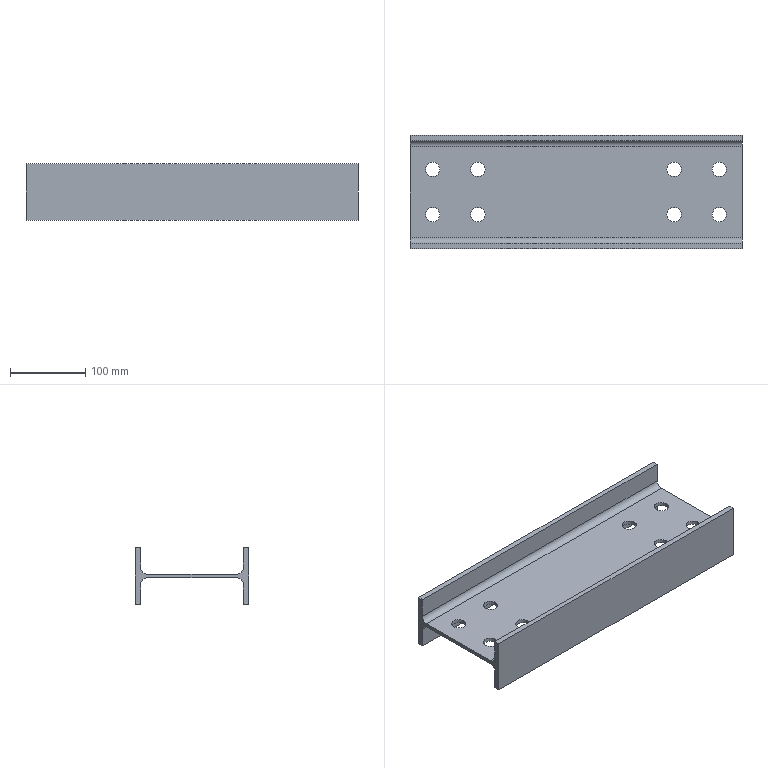Part | STEP file | 粉仓辅梁5_Default<As Machined> | 1 solid | 34 faces | box 440 x 150 x 75 mm | volume 774032 mm3 | cylinder 20 | plane 14 | commonest cylinder face diameters 19 x16 16 x4